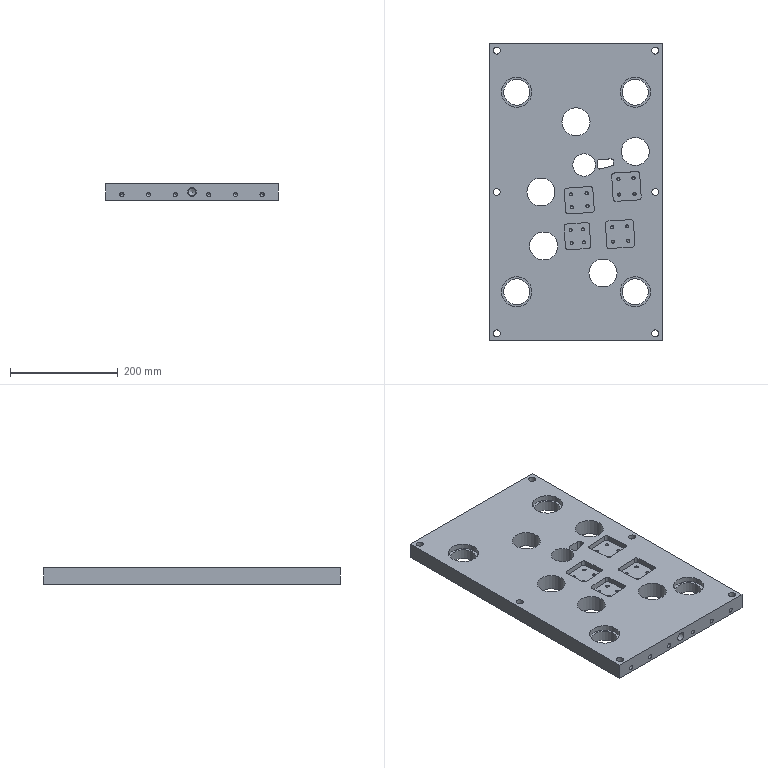Part | STEP file | 车灯-后视镜_id38_x_t | 1 solid | 214 faces | box 320 x 550 x 30 mm | volume 4485754 mm3 | cylinder 110 | plane 67 | cone 34 | spline 3 | commonest cylinder face diameters 5.1 x16 6 x16 8 x16 10 x16 6.9 x8 13 x6